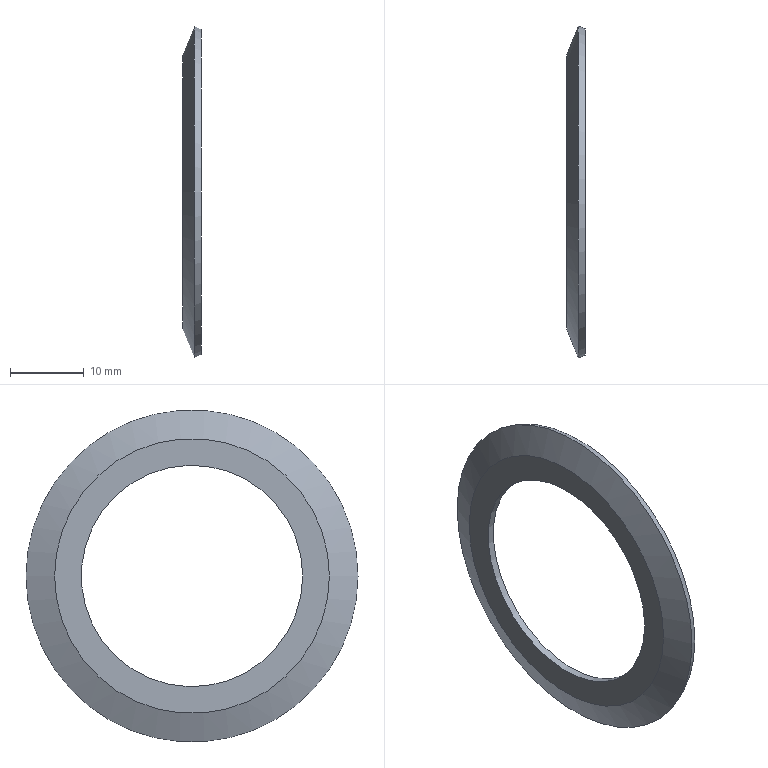Part | NX | features Flange_5003_015_HTLA24S5M150-E-10 2 | 1 solid | 6 faces | box 2.495 x 45 x 45 mm | volume 895.426 mm3 | cone 3 | plane 2 | cylinder 1 | commonest cylinder face diameters 30 x1
STEP:
#1=CARTESIAN_POINT('',(215.025,105.38,-147.));
#2=VERTEX_POINT('',#1);
#3=CARTESIAN_POINT('',(215.025,124.,-147.));
#4=DIRECTION('',(-1.,0.,0.));
#5=DIRECTION('',(0.,-1.,0.));
#6=AXIS2_PLACEMENT_3D('',#3,#4,#5);
#7=CIRCLE('',#6,18.62);
#8=EDGE_CURVE('',#2,#2,#7,.T.);
#9=ORIENTED_EDGE('',*,*,#8,.F.);
#10=EDGE_LOOP('',(#9));
#11=FACE_BOUND('',#10,.T.);
#12=CARTESIAN_POINT('',(216.593,101.5,-147.));
#13=VERTEX_POINT('',#12);
#14=CARTESIAN_POINT('',(216.593,124.,-147.));
#15=DIRECTION('',(-1.,0.,0.));
#16=DIRECTION('',(0.,-1.,0.));
#17=AXIS2_PLACEMENT_3D('',#14,#15,#16);
#18=CIRCLE('',#17,22.5);
#19=EDGE_CURVE('',#13,#13,#18,.T.);
#20=ORIENTED_EDGE('',*,*,#19,.T.);
#21=EDGE_LOOP('',(#20));
#22=FACE_BOUND('',#21,.T.);
#23=CARTESIAN_POINT('',(216.593,124.,-147.));
#24=DIRECTION('',(1.,0.,0.));
#25=DIRECTION('',(0.,1.,0.));
#26=AXIS2_PLACEMENT_3D('',#23,#24,#25);
#27=CONICAL_SURFACE('',#26,22.5,1.187);
#28=ADVANCED_FACE('',(#11,#22),#27,.T.);
#29=ORIENTED_EDGE('',*,*,#19,.F.);
#30=EDGE_LOOP('',(#29));
#31=FACE_BOUND('',#30,.T.);
#32=CARTESIAN_POINT('',(217.52,101.875,-147.));
#33=VERTEX_POINT('',#32);
#34=CARTESIAN_POINT('',(217.52,124.,-147.));
#35=DIRECTION('',(-1.,0.,0.));
#36=DIRECTION('',(0.,-1.,0.));
#37=AXIS2_PLACEMENT_3D('',#34,#35,#36);
#38=CIRCLE('',#37,22.125);
#39=EDGE_CURVE('',#33,#33,#38,.T.);
#40=ORIENTED_EDGE('',*,*,#39,.T.);
#41=EDGE_LOOP('',(#40));
#42=FACE_BOUND('',#41,.T.);
#43=CARTESIAN_POINT('',(217.52,124.,-147.));
#44=DIRECTION('',(-1.,0.,0.));
#45=DIRECTION('',(0.,-1.,0.));
#46=AXIS2_PLACEMENT_3D('',#43,#44,#45);
#47=CONICAL_SURFACE('',#46,22.125,0.384);
#48=ADVANCED_FACE('',(#31,#42),#47,.T.);
#49=ORIENTED_EDGE('',*,*,#39,.F.);
#50=EDGE_LOOP('',(#49));
#51=FACE_BOUND('',#50,.T.);
#52=CARTESIAN_POINT('',(216.025,105.574,-147.));
#53=VERTEX_POINT('',#52);
#54=CARTESIAN_POINT('',(216.025,124.,-147.));
#55=DIRECTION('',(-1.,0.,0.));
#56=DIRECTION('',(0.,-1.,0.));
#57=AXIS2_PLACEMENT_3D('',#54,#55,#56);
#58=CIRCLE('',#57,18.426);
#59=EDGE_CURVE('',#53,#53,#58,.T.);
#60=ORIENTED_EDGE('',*,*,#59,.T.);
#61=EDGE_LOOP('',(#60));
#62=FACE_BOUND('',#61,.T.);
#63=CARTESIAN_POINT('',(216.025,124.,-147.));
#64=DIRECTION('',(1.,0.,0.));
#65=DIRECTION('',(0.,1.,0.));
#66=AXIS2_PLACEMENT_3D('',#63,#64,#65);
#67=CONICAL_SURFACE('',#66,18.426,1.187);
#68=ADVANCED_FACE('',(#51,#62),#67,.F.);
#69=ORIENTED_EDGE('',*,*,#59,.F.);
#70=EDGE_LOOP('',(#69));
#71=FACE_BOUND('',#70,.T.);
#72=CARTESIAN_POINT('',(216.025,109.,-147.));
#73=VERTEX_POINT('',#72);
#74=CARTESIAN_POINT('',(216.025,124.,-147.));
#75=DIRECTION('',(-1.,0.,0.));
#76=DIRECTION('',(0.,-1.,0.));
#77=AXIS2_PLACEMENT_3D('',#74,#75,#76);
#78=CIRCLE('',#77,15.);
#79=EDGE_CURVE('',#73,#73,#78,.T.);
#80=ORIENTED_EDGE('',*,*,#79,.T.);
#81=EDGE_LOOP('',(#80));
#82=FACE_BOUND('',#81,.T.);
#83=CARTESIAN_POINT('',(216.025,124.,-132.));
#84=DIRECTION('',(-1.,0.,0.));
#85=DIRECTION('',(0.,-1.,0.));
#86=AXIS2_PLACEMENT_3D('',#83,#84,#85);
#87=PLANE('',#86);
#88=ADVANCED_FACE('',(#71,#82),#87,.F.);
#89=ORIENTED_EDGE('',*,*,#79,.F.);
#90=EDGE_LOOP('',(#89));
#91=FACE_BOUND('',#90,.T.);
#92=CARTESIAN_POINT('',(215.025,109.,-147.));
#93=VERTEX_POINT('',#92);
#94=CARTESIAN_POINT('',(215.025,124.,-147.));
#95=DIRECTION('',(-1.,0.,0.));
#96=DIRECTION('',(0.,-1.,0.));
#97=AXIS2_PLACEMENT_3D('',#94,#95,#96);
#98=CIRCLE('',#97,15.);
#99=EDGE_CURVE('',#93,#93,#98,.T.);
#100=ORIENTED_EDGE('',*,*,#99,.T.);
#101=EDGE_LOOP('',(#100));
#102=FACE_BOUND('',#101,.T.);
#103=CARTESIAN_POINT('',(215.025,124.,-147.));
#104=DIRECTION('',(-1.,0.,0.));
#105=DIRECTION('',(0.,-1.,0.));
#106=AXIS2_PLACEMENT_3D('',#103,#104,#105);
#107=CYLINDRICAL_SURFACE('',#106,15.);
#108=ADVANCED_FACE('',(#91,#102),#107,.F.);
#109=ORIENTED_EDGE('',*,*,#99,.F.);
#110=EDGE_LOOP('',(#109));
#111=FACE_BOUND('',#110,.T.);
#112=ORIENTED_EDGE('',*,*,#8,.T.);
#113=EDGE_LOOP('',(#112));
#114=FACE_BOUND('',#113,.T.);
#115=CARTESIAN_POINT('',(215.025,124.,-128.38));
#116=DIRECTION('',(1.,0.,0.));
#117=DIRECTION('',(0.,1.,0.));
#118=AXIS2_PLACEMENT_3D('',#115,#116,#117);
#119=PLANE('',#118);
#120=ADVANCED_FACE('',(#111,#114),#119,.F.);
#121=CLOSED_SHELL('',(#28,#48,#68,#88,#108,#120));
#122=MANIFOLD_SOLID_BREP('',#121);
#123=(LENGTH_UNIT()NAMED_UNIT(*)SI_UNIT(.MILLI.,.METRE.));
#124=UNCERTAINTY_MEASURE_WITH_UNIT(LENGTH_MEASURE(0.00001),#123,'','');
#125=(NAMED_UNIT(*)PLANE_ANGLE_UNIT()SI_UNIT($,.RADIAN.));
#126=(NAMED_UNIT(*)SI_UNIT($,.STERADIAN.)SOLID_ANGLE_UNIT());
#127=(GEOMETRIC_REPRESENTATION_CONTEXT(3)GLOBAL_UNCERTAINTY_ASSIGNED_CONTEXT((#124))GLOBAL_UNIT_ASSIGNED_CONTEXT((#123,#125,#126))REPRESENTATION_CONTEXT('',''));
#128=ADVANCED_BREP_SHAPE_REPRESENTATION('',(#122),#127);